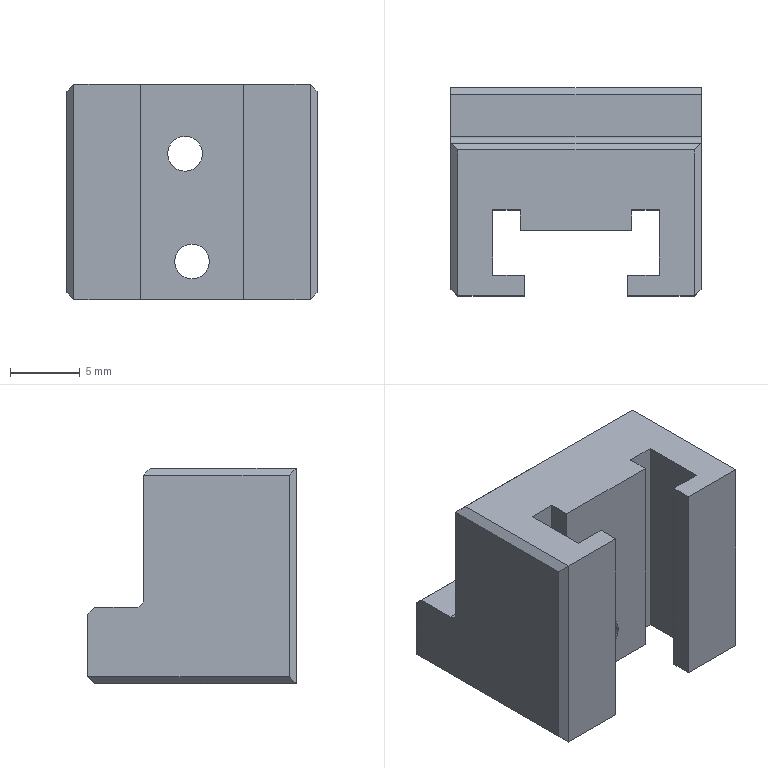Part | SolidWorks | features HoleWzd 2, Chamfer 1, Cut 1, Extrusion 1, Fillet 1 | 1 solid | 34 faces | box 18 x 15 x 15.5 mm | volume 2507 mm3 | plane 29 | cylinder 5 | commonest cylinder face diameters 2.5 x4 1 x1
STEP:
#1=CARTESIAN_POINT('',(0.,0.,-25.5));
#2=VERTEX_POINT('',#1);
#3=CARTESIAN_POINT('',(0.,0.,-28.));
#4=VERTEX_POINT('',#3);
#5=CARTESIAN_POINT('',(0.,0.,-26.75));
#6=DIRECTION('',(0.,-1.,0.));
#7=DIRECTION('',(1.,0.,0.));
#8=AXIS2_PLACEMENT_3D('',#5,#6,#7);
#9=CIRCLE('',#8,1.25);
#10=EDGE_CURVE('',#2,#4,#9,.T.);
#11=ORIENTED_EDGE('',*,*,#10,.T.);
#12=CARTESIAN_POINT('',(0.,10.3,-28.));
#13=VERTEX_POINT('',#12);
#14=CARTESIAN_POINT('',(0.,10.3,-28.));
#15=DIRECTION('',(0.,1.,0.));
#16=VECTOR('',#15,1000.);
#17=LINE('',#14,#16);
#18=EDGE_CURVE('',#4,#13,#17,.T.);
#19=ORIENTED_EDGE('',*,*,#18,.T.);
#20=CARTESIAN_POINT('',(0.,10.3,-25.5));
#21=VERTEX_POINT('',#20);
#22=CARTESIAN_POINT('',(0.,10.3,-26.75));
#23=DIRECTION('',(0.,1.,0.));
#24=DIRECTION('',(0.,0.,1.));
#25=AXIS2_PLACEMENT_3D('',#22,#23,#24);
#26=CIRCLE('',#25,1.25);
#27=EDGE_CURVE('',#13,#21,#26,.T.);
#28=ORIENTED_EDGE('',*,*,#27,.T.);
#29=CARTESIAN_POINT('',(0.,10.3,-25.5));
#30=DIRECTION('',(0.,1.,0.));
#31=VECTOR('',#30,1000.);
#32=LINE('',#29,#31);
#33=EDGE_CURVE('',#2,#21,#32,.T.);
#34=ORIENTED_EDGE('',*,*,#33,.F.);
#35=EDGE_LOOP('',(#11,#19,#28,#34));
#36=FACE_OUTER_BOUND('',#35,.T.);
#37=CARTESIAN_POINT('',(0.,10.3,-26.75));
#38=DIRECTION('',(0.,1.,0.));
#39=DIRECTION('',(0.,0.,1.));
#40=AXIS2_PLACEMENT_3D('',#37,#38,#39);
#41=CYLINDRICAL_SURFACE('',#40,1.25);
#42=ADVANCED_FACE('',(#36),#41,.F.);
#43=CARTESIAN_POINT('',(-0.5,0.,-17.75));
#44=VERTEX_POINT('',#43);
#45=CARTESIAN_POINT('',(-0.5,0.,-20.25));
#46=VERTEX_POINT('',#45);
#47=CARTESIAN_POINT('',(-0.5,0.,-19.));
#48=DIRECTION('',(0.,-1.,0.));
#49=DIRECTION('',(1.,0.,0.));
#50=AXIS2_PLACEMENT_3D('',#47,#48,#49);
#51=CIRCLE('',#50,1.25);
#52=EDGE_CURVE('',#44,#46,#51,.T.);
#53=ORIENTED_EDGE('',*,*,#52,.T.);
#54=CARTESIAN_POINT('',(-0.5,6.3,-20.25));
#55=VERTEX_POINT('',#54);
#56=CARTESIAN_POINT('',(-0.5,6.3,-20.25));
#57=DIRECTION('',(0.,1.,0.));
#58=VECTOR('',#57,1000.);
#59=LINE('',#56,#58);
#60=EDGE_CURVE('',#46,#55,#59,.T.);
#61=ORIENTED_EDGE('',*,*,#60,.T.);
#62=CARTESIAN_POINT('',(-0.5,6.3,-17.75));
#63=VERTEX_POINT('',#62);
#64=CARTESIAN_POINT('',(-0.5,6.3,-19.));
#65=DIRECTION('',(0.,1.,0.));
#66=DIRECTION('',(0.,0.,1.));
#67=AXIS2_PLACEMENT_3D('',#64,#65,#66);
#68=CIRCLE('',#67,1.25);
#69=EDGE_CURVE('',#55,#63,#68,.T.);
#70=ORIENTED_EDGE('',*,*,#69,.T.);
#71=CARTESIAN_POINT('',(-0.5,6.3,-17.75));
#72=DIRECTION('',(0.,1.,0.));
#73=VECTOR('',#72,1000.);
#74=LINE('',#71,#73);
#75=EDGE_CURVE('',#44,#63,#74,.T.);
#76=ORIENTED_EDGE('',*,*,#75,.F.);
#77=EDGE_LOOP('',(#53,#61,#70,#76));
#78=FACE_OUTER_BOUND('',#77,.T.);
#79=CARTESIAN_POINT('',(-0.5,6.3,-19.));
#80=DIRECTION('',(0.,1.,0.));
#81=DIRECTION('',(0.,0.,1.));
#82=AXIS2_PLACEMENT_3D('',#79,#80,#81);
#83=CYLINDRICAL_SURFACE('',#82,1.25);
#84=ADVANCED_FACE('',(#78),#83,.F.);
#85=CARTESIAN_POINT('',(3.7,-4.7,-29.5));
#86=VERTEX_POINT('',#85);
#87=CARTESIAN_POINT('',(8.5,-4.7,-29.5));
#88=VERTEX_POINT('',#87);
#89=CARTESIAN_POINT('',(3.7,-4.7,-29.5));
#90=DIRECTION('',(1.,0.,0.));
#91=VECTOR('',#90,1000.);
#92=LINE('',#89,#91);
#93=EDGE_CURVE('',#86,#88,#92,.T.);
#94=ORIENTED_EDGE('',*,*,#93,.T.);
#95=CARTESIAN_POINT('',(8.5,-4.7,-14.));
#96=VERTEX_POINT('',#95);
#97=CARTESIAN_POINT('',(8.5,-4.7,-29.5));
#98=DIRECTION('',(0.,0.,1.));
#99=VECTOR('',#98,1000.);
#100=LINE('',#97,#99);
#101=EDGE_CURVE('',#88,#96,#100,.T.);
#102=ORIENTED_EDGE('',*,*,#101,.T.);
#103=CARTESIAN_POINT('',(3.7,-4.7,-14.));
#104=VERTEX_POINT('',#103);
#105=CARTESIAN_POINT('',(3.7,-4.7,-14.));
#106=DIRECTION('',(1.,0.,0.));
#107=VECTOR('',#106,1000.);
#108=LINE('',#105,#107);
#109=EDGE_CURVE('',#104,#96,#108,.T.);
#110=ORIENTED_EDGE('',*,*,#109,.F.);
#111=CARTESIAN_POINT('',(3.7,-4.7,-29.5));
#112=DIRECTION('',(0.,0.,1.));
#113=VECTOR('',#112,1000.);
#114=LINE('',#111,#113);
#115=EDGE_CURVE('',#86,#104,#114,.T.);
#116=ORIENTED_EDGE('',*,*,#115,.F.);
#117=EDGE_LOOP('',(#94,#102,#110,#116));
#118=FACE_OUTER_BOUND('',#117,.T.);
#119=CARTESIAN_POINT('',(3.7,-4.7,-29.5));
#120=DIRECTION('',(0.,-1.,0.));
#121=DIRECTION('',(1.,0.,0.));
#122=AXIS2_PLACEMENT_3D('',#119,#120,#121);
#123=PLANE('',#122);
#124=ADVANCED_FACE('',(#118),#123,.T.);
#125=CARTESIAN_POINT('',(3.7,-3.2,-14.));
#126=VERTEX_POINT('',#125);
#127=CARTESIAN_POINT('',(3.7,-3.2,-14.));
#128=DIRECTION('',(0.,-1.,0.));
#129=VECTOR('',#128,1000.);
#130=LINE('',#127,#129);
#131=EDGE_CURVE('',#126,#104,#130,.T.);
#132=ORIENTED_EDGE('',*,*,#131,.F.);
#133=CARTESIAN_POINT('',(3.7,-3.2,-29.5));
#134=VERTEX_POINT('',#133);
#135=CARTESIAN_POINT('',(3.7,-3.2,-29.5));
#136=DIRECTION('',(0.,0.,1.));
#137=VECTOR('',#136,1000.);
#138=LINE('',#135,#137);
#139=EDGE_CURVE('',#134,#126,#138,.T.);
#140=ORIENTED_EDGE('',*,*,#139,.F.);
#141=CARTESIAN_POINT('',(3.7,-3.2,-29.5));
#142=DIRECTION('',(0.,-1.,0.));
#143=VECTOR('',#142,1000.);
#144=LINE('',#141,#143);
#145=EDGE_CURVE('',#134,#86,#144,.T.);
#146=ORIENTED_EDGE('',*,*,#145,.T.);
#147=ORIENTED_EDGE('',*,*,#115,.T.);
#148=EDGE_LOOP('',(#132,#140,#146,#147));
#149=FACE_OUTER_BOUND('',#148,.T.);
#150=CARTESIAN_POINT('',(3.7,-3.2,-29.5));
#151=DIRECTION('',(-1.,0.,0.));
#152=DIRECTION('',(0.,0.,1.));
#153=AXIS2_PLACEMENT_3D('',#150,#151,#152);
#154=PLANE('',#153);
#155=ADVANCED_FACE('',(#149),#154,.T.);
#156=CARTESIAN_POINT('',(6.,-3.2,-14.));
#157=VERTEX_POINT('',#156);
#158=CARTESIAN_POINT('',(6.,-3.2,-14.));
#159=DIRECTION('',(-1.,0.,0.));
#160=VECTOR('',#159,1000.);
#161=LINE('',#158,#160);
#162=EDGE_CURVE('',#157,#126,#161,.T.);
#163=ORIENTED_EDGE('',*,*,#162,.F.);
#164=CARTESIAN_POINT('',(6.,-3.2,-29.5));
#165=VERTEX_POINT('',#164);
#166=CARTESIAN_POINT('',(6.,-3.2,-29.5));
#167=DIRECTION('',(0.,0.,1.));
#168=VECTOR('',#167,1000.);
#169=LINE('',#166,#168);
#170=EDGE_CURVE('',#165,#157,#169,.T.);
#171=ORIENTED_EDGE('',*,*,#170,.F.);
#172=CARTESIAN_POINT('',(6.,-3.2,-29.5));
#173=DIRECTION('',(-1.,0.,0.));
#174=VECTOR('',#173,1000.);
#175=LINE('',#172,#174);
#176=EDGE_CURVE('',#165,#134,#175,.T.);
#177=ORIENTED_EDGE('',*,*,#176,.T.);
#178=ORIENTED_EDGE('',*,*,#139,.T.);
#179=EDGE_LOOP('',(#163,#171,#177,#178));
#180=FACE_OUTER_BOUND('',#179,.T.);
#181=CARTESIAN_POINT('',(6.,-3.2,-29.5));
#182=DIRECTION('',(0.,1.,0.));
#183=DIRECTION('',(0.,0.,1.));
#184=AXIS2_PLACEMENT_3D('',#181,#182,#183);
#185=PLANE('',#184);
#186=ADVANCED_FACE('',(#180),#185,.T.);
#187=CARTESIAN_POINT('',(6.,1.5,-14.));
#188=VERTEX_POINT('',#187);
#189=CARTESIAN_POINT('',(6.,1.5,-14.));
#190=DIRECTION('',(0.,-1.,0.));
#191=VECTOR('',#190,1000.);
#192=LINE('',#189,#191);
#193=EDGE_CURVE('',#188,#157,#192,.T.);
#194=ORIENTED_EDGE('',*,*,#193,.F.);
#195=CARTESIAN_POINT('',(6.,1.5,-29.5));
#196=VERTEX_POINT('',#195);
#197=CARTESIAN_POINT('',(6.,1.5,-29.5));
#198=DIRECTION('',(0.,0.,1.));
#199=VECTOR('',#198,1000.);
#200=LINE('',#197,#199);
#201=EDGE_CURVE('',#196,#188,#200,.T.);
#202=ORIENTED_EDGE('',*,*,#201,.F.);
#203=CARTESIAN_POINT('',(6.,1.5,-29.5));
#204=DIRECTION('',(0.,-1.,0.));
#205=VECTOR('',#204,1000.);
#206=LINE('',#203,#205);
#207=EDGE_CURVE('',#196,#165,#206,.T.);
#208=ORIENTED_EDGE('',*,*,#207,.T.);
#209=ORIENTED_EDGE('',*,*,#170,.T.);
#210=EDGE_LOOP('',(#194,#202,#208,#209));
#211=FACE_OUTER_BOUND('',#210,.T.);
#212=CARTESIAN_POINT('',(6.,1.5,-29.5));
#213=DIRECTION('',(-1.,0.,0.));
#214=DIRECTION('',(0.,-1.,0.));
#215=AXIS2_PLACEMENT_3D('',#212,#213,#214);
#216=PLANE('',#215);
#217=ADVANCED_FACE('',(#211),#216,.T.);
#218=CARTESIAN_POINT('',(4.,1.5,-14.));
#219=VERTEX_POINT('',#218);
#220=CARTESIAN_POINT('',(4.,1.5,-14.));
#221=DIRECTION('',(1.,0.,0.));
#222=VECTOR('',#221,1000.);
#223=LINE('',#220,#222);
#224=EDGE_CURVE('',#219,#188,#223,.T.);
#225=ORIENTED_EDGE('',*,*,#224,.F.);
#226=CARTESIAN_POINT('',(4.,1.5,-29.5));
#227=VERTEX_POINT('',#226);
#228=CARTESIAN_POINT('',(4.,1.5,-29.5));
#229=DIRECTION('',(0.,0.,1.));
#230=VECTOR('',#229,1000.);
#231=LINE('',#228,#230);
#232=EDGE_CURVE('',#227,#219,#231,.T.);
#233=ORIENTED_EDGE('',*,*,#232,.F.);
#234=CARTESIAN_POINT('',(4.,1.5,-29.5));
#235=DIRECTION('',(1.,0.,0.));
#236=VECTOR('',#235,1000.);
#237=LINE('',#234,#236);
#238=EDGE_CURVE('',#227,#196,#237,.T.);
#239=ORIENTED_EDGE('',*,*,#238,.T.);
#240=ORIENTED_EDGE('',*,*,#201,.T.);
#241=EDGE_LOOP('',(#225,#233,#239,#240));
#242=FACE_OUTER_BOUND('',#241,.T.);
#243=CARTESIAN_POINT('',(4.,1.5,-29.5));
#244=DIRECTION('',(0.,-1.,0.));
#245=DIRECTION('',(0.,0.,-1.));
#246=AXIS2_PLACEMENT_3D('',#243,#244,#245);
#247=PLANE('',#246);
#248=ADVANCED_FACE('',(#242),#247,.T.);
#249=CARTESIAN_POINT('',(4.,0.,-14.));
#250=VERTEX_POINT('',#249);
#251=CARTESIAN_POINT('',(4.,0.,-14.));
#252=DIRECTION('',(0.,1.,0.));
#253=VECTOR('',#252,1000.);
#254=LINE('',#251,#253);
#255=EDGE_CURVE('',#250,#219,#254,.T.);
#256=ORIENTED_EDGE('',*,*,#255,.F.);
#257=CARTESIAN_POINT('',(4.,0.,-29.5));
#258=VERTEX_POINT('',#257);
#259=CARTESIAN_POINT('',(4.,0.,-29.5));
#260=DIRECTION('',(0.,0.,1.));
#261=VECTOR('',#260,1000.);
#262=LINE('',#259,#261);
#263=EDGE_CURVE('',#258,#250,#262,.T.);
#264=ORIENTED_EDGE('',*,*,#263,.F.);
#265=CARTESIAN_POINT('',(4.,0.,-29.5));
#266=DIRECTION('',(0.,1.,0.));
#267=VECTOR('',#266,1000.);
#268=LINE('',#265,#267);
#269=EDGE_CURVE('',#258,#227,#268,.T.);
#270=ORIENTED_EDGE('',*,*,#269,.T.);
#271=ORIENTED_EDGE('',*,*,#232,.T.);
#272=EDGE_LOOP('',(#256,#264,#270,#271));
#273=FACE_OUTER_BOUND('',#272,.T.);
#274=CARTESIAN_POINT('',(4.,0.,-29.5));
#275=DIRECTION('',(1.,0.,0.));
#276=DIRECTION('',(0.,1.,0.));
#277=AXIS2_PLACEMENT_3D('',#274,#275,#276);
#278=PLANE('',#277);
#279=ADVANCED_FACE('',(#273),#278,.T.);
#280=ORIENTED_EDGE('',*,*,#10,.F.);
#281=CARTESIAN_POINT('',(0.,0.,-26.75));
#282=DIRECTION('',(0.,-1.,0.));
#283=DIRECTION('',(1.,0.,0.));
#284=AXIS2_PLACEMENT_3D('',#281,#282,#283);
#285=CIRCLE('',#284,1.25);
#286=EDGE_CURVE('',#4,#2,#285,.T.);
#287=ORIENTED_EDGE('',*,*,#286,.F.);
#288=EDGE_LOOP('',(#280,#287));
#289=FACE_BOUND('',#288,.T.);
#290=ORIENTED_EDGE('',*,*,#52,.F.);
#291=CARTESIAN_POINT('',(-0.5,0.,-19.));
#292=DIRECTION('',(0.,-1.,0.));
#293=DIRECTION('',(1.,0.,0.));
#294=AXIS2_PLACEMENT_3D('',#291,#292,#293);
#295=CIRCLE('',#294,1.25);
#296=EDGE_CURVE('',#46,#44,#295,.T.);
#297=ORIENTED_EDGE('',*,*,#296,.F.);
#298=EDGE_LOOP('',(#290,#297));
#299=FACE_BOUND('',#298,.T.);
#300=CARTESIAN_POINT('',(-4.,0.,-14.));
#301=VERTEX_POINT('',#300);
#302=CARTESIAN_POINT('',(0.,0.,-14.));
#303=DIRECTION('',(1.,0.,0.));
#304=VECTOR('',#303,1000.);
#305=LINE('',#302,#304);
#306=EDGE_CURVE('',#301,#250,#305,.T.);
#307=ORIENTED_EDGE('',*,*,#306,.F.);
#308=CARTESIAN_POINT('',(-4.,0.,-29.5));
#309=VERTEX_POINT('',#308);
#310=CARTESIAN_POINT('',(-4.,0.,-29.5));
#311=DIRECTION('',(0.,0.,1.));
#312=VECTOR('',#311,1000.);
#313=LINE('',#310,#312);
#314=EDGE_CURVE('',#309,#301,#313,.T.);
#315=ORIENTED_EDGE('',*,*,#314,.F.);
#316=CARTESIAN_POINT('',(-4.,0.,-29.5));
#317=DIRECTION('',(1.,0.,0.));
#318=VECTOR('',#317,1000.);
#319=LINE('',#316,#318);
#320=EDGE_CURVE('',#309,#258,#319,.T.);
#321=ORIENTED_EDGE('',*,*,#320,.T.);
#322=ORIENTED_EDGE('',*,*,#263,.T.);
#323=EDGE_LOOP('',(#307,#315,#321,#322));
#324=FACE_OUTER_BOUND('',#323,.T.);
#325=CARTESIAN_POINT('',(0.,0.,-29.5));
#326=DIRECTION('',(0.,-1.,0.));
#327=DIRECTION('',(1.,0.,0.));
#328=AXIS2_PLACEMENT_3D('',#325,#326,#327);
#329=PLANE('',#328);
#330=ADVANCED_FACE('',(#289,#299,#324),#329,.T.);
#331=CARTESIAN_POINT('',(-4.,1.5,-14.));
#332=VERTEX_POINT('',#331);
#333=CARTESIAN_POINT('',(-4.,1.5,-14.));
#334=DIRECTION('',(0.,-1.,0.));
#335=VECTOR('',#334,1000.);
#336=LINE('',#333,#335);
#337=EDGE_CURVE('',#332,#301,#336,.T.);
#338=ORIENTED_EDGE('',*,*,#337,.F.);
#339=CARTESIAN_POINT('',(-4.,1.5,-29.5));
#340=VERTEX_POINT('',#339);
#341=CARTESIAN_POINT('',(-4.,1.5,-29.5));
#342=DIRECTION('',(0.,0.,1.));
#343=VECTOR('',#342,1000.);
#344=LINE('',#341,#343);
#345=EDGE_CURVE('',#340,#332,#344,.T.);
#346=ORIENTED_EDGE('',*,*,#345,.F.);
#347=CARTESIAN_POINT('',(-4.,1.5,-29.5));
#348=DIRECTION('',(0.,-1.,0.));
#349=VECTOR('',#348,1000.);
#350=LINE('',#347,#349);
#351=EDGE_CURVE('',#340,#309,#350,.T.);
#352=ORIENTED_EDGE('',*,*,#351,.T.);
#353=ORIENTED_EDGE('',*,*,#314,.T.);
#354=EDGE_LOOP('',(#338,#346,#352,#353));
#355=FACE_OUTER_BOUND('',#354,.T.);
#356=CARTESIAN_POINT('',(-4.,1.5,-29.5));
#357=DIRECTION('',(-1.,0.,0.));
#358=DIRECTION('',(0.,-1.,0.));
#359=AXIS2_PLACEMENT_3D('',#356,#357,#358);
#360=PLANE('',#359);
#361=ADVANCED_FACE('',(#355),#360,.T.);
#362=CARTESIAN_POINT('',(-6.,1.5,-14.));
#363=VERTEX_POINT('',#362);
#364=CARTESIAN_POINT('',(-6.,1.5,-14.));
#365=DIRECTION('',(1.,0.,0.));
#366=VECTOR('',#365,1000.);
#367=LINE('',#364,#366);
#368=EDGE_CURVE('',#363,#332,#367,.T.);
#369=ORIENTED_EDGE('',*,*,#368,.F.);
#370=CARTESIAN_POINT('',(-6.,1.5,-29.5));
#371=VERTEX_POINT('',#370);
#372=CARTESIAN_POINT('',(-6.,1.5,-29.5));
#373=DIRECTION('',(0.,0.,1.));
#374=VECTOR('',#373,1000.);
#375=LINE('',#372,#374);
#376=EDGE_CURVE('',#371,#363,#375,.T.);
#377=ORIENTED_EDGE('',*,*,#376,.F.);
#378=CARTESIAN_POINT('',(-6.,1.5,-29.5));
#379=DIRECTION('',(1.,0.,0.));
#380=VECTOR('',#379,1000.);
#381=LINE('',#378,#380);
#382=EDGE_CURVE('',#371,#340,#381,.T.);
#383=ORIENTED_EDGE('',*,*,#382,.T.);
#384=ORIENTED_EDGE('',*,*,#345,.T.);
#385=EDGE_LOOP('',(#369,#377,#383,#384));
#386=FACE_OUTER_BOUND('',#385,.T.);
#387=CARTESIAN_POINT('',(-6.,1.5,-29.5));
#388=DIRECTION('',(0.,-1.,0.));
#389=DIRECTION('',(0.,0.,-1.));
#390=AXIS2_PLACEMENT_3D('',#387,#388,#389);
#391=PLANE('',#390);
#392=ADVANCED_FACE('',(#386),#391,.T.);
#393=CARTESIAN_POINT('',(-6.,-3.2,-14.));
#394=VERTEX_POINT('',#393);
#395=CARTESIAN_POINT('',(-6.,-3.2,-14.));
#396=DIRECTION('',(0.,1.,0.));
#397=VECTOR('',#396,1000.);
#398=LINE('',#395,#397);
#399=EDGE_CURVE('',#394,#363,#398,.T.);
#400=ORIENTED_EDGE('',*,*,#399,.F.);
#401=CARTESIAN_POINT('',(-6.,-3.2,-29.5));
#402=VERTEX_POINT('',#401);
#403=CARTESIAN_POINT('',(-6.,-3.2,-29.5));
#404=DIRECTION('',(0.,0.,1.));
#405=VECTOR('',#404,1000.);
#406=LINE('',#403,#405);
#407=EDGE_CURVE('',#402,#394,#406,.T.);
#408=ORIENTED_EDGE('',*,*,#407,.F.);
#409=CARTESIAN_POINT('',(-6.,-3.2,-29.5));
#410=DIRECTION('',(0.,1.,0.));
#411=VECTOR('',#410,1000.);
#412=LINE('',#409,#411);
#413=EDGE_CURVE('',#402,#371,#412,.T.);
#414=ORIENTED_EDGE('',*,*,#413,.T.);
#415=ORIENTED_EDGE('',*,*,#376,.T.);
#416=EDGE_LOOP('',(#400,#408,#414,#415));
#417=FACE_OUTER_BOUND('',#416,.T.);
#418=CARTESIAN_POINT('',(-6.,-3.2,-29.5));
#419=DIRECTION('',(1.,0.,0.));
#420=DIRECTION('',(0.,1.,0.));
#421=AXIS2_PLACEMENT_3D('',#418,#419,#420);
#422=PLANE('',#421);
#423=ADVANCED_FACE('',(#417),#422,.T.);
#424=CARTESIAN_POINT('',(-3.7,-3.2,-14.));
#425=VERTEX_POINT('',#424);
#426=CARTESIAN_POINT('',(-3.7,-3.2,-14.));
#427=DIRECTION('',(-1.,0.,0.));
#428=VECTOR('',#427,1000.);
#429=LINE('',#426,#428);
#430=EDGE_CURVE('',#425,#394,#429,.T.);
#431=ORIENTED_EDGE('',*,*,#430,.F.);
#432=CARTESIAN_POINT('',(-3.7,-3.2,-29.5));
#433=VERTEX_POINT('',#432);
#434=CARTESIAN_POINT('',(-3.7,-3.2,-29.5));
#435=DIRECTION('',(0.,0.,1.));
#436=VECTOR('',#435,1000.);
#437=LINE('',#434,#436);
#438=EDGE_CURVE('',#433,#425,#437,.T.);
#439=ORIENTED_EDGE('',*,*,#438,.F.);
#440=CARTESIAN_POINT('',(-3.7,-3.2,-29.5));
#441=DIRECTION('',(-1.,0.,0.));
#442=VECTOR('',#441,1000.);
#443=LINE('',#440,#442);
#444=EDGE_CURVE('',#433,#402,#443,.T.);
#445=ORIENTED_EDGE('',*,*,#444,.T.);
#446=ORIENTED_EDGE('',*,*,#407,.T.);
#447=EDGE_LOOP('',(#431,#439,#445,#446));
#448=FACE_OUTER_BOUND('',#447,.T.);
#449=CARTESIAN_POINT('',(-3.7,-3.2,-29.5));
#450=DIRECTION('',(0.,1.,0.));
#451=DIRECTION('',(0.,0.,1.));
#452=AXIS2_PLACEMENT_3D('',#449,#450,#451);
#453=PLANE('',#452);
#454=ADVANCED_FACE('',(#448),#453,.T.);
#455=CARTESIAN_POINT('',(-3.7,-4.7,-14.));
#456=VERTEX_POINT('',#455);
#457=CARTESIAN_POINT('',(-3.7,-3.2,-14.));
#458=DIRECTION('',(0.,-1.,0.));
#459=VECTOR('',#458,1000.);
#460=LINE('',#457,#459);
#461=EDGE_CURVE('',#425,#456,#460,.T.);
#462=ORIENTED_EDGE('',*,*,#461,.T.);
#463=CARTESIAN_POINT('',(-3.7,-4.7,-29.5));
#464=VERTEX_POINT('',#463);
#465=CARTESIAN_POINT('',(-3.7,-4.7,-29.5));
#466=DIRECTION('',(0.,0.,1.));
#467=VECTOR('',#466,1000.);
#468=LINE('',#465,#467);
#469=EDGE_CURVE('',#464,#456,#468,.T.);
#470=ORIENTED_EDGE('',*,*,#469,.F.);
#471=CARTESIAN_POINT('',(-3.7,-3.2,-29.5));
#472=DIRECTION('',(0.,-1.,0.));
#473=VECTOR('',#472,1000.);
#474=LINE('',#471,#473);
#475=EDGE_CURVE('',#433,#464,#474,.T.);
#476=ORIENTED_EDGE('',*,*,#475,.F.);
#477=ORIENTED_EDGE('',*,*,#438,.T.);
#478=EDGE_LOOP('',(#462,#470,#476,#477));
#479=FACE_OUTER_BOUND('',#478,.T.);
#480=CARTESIAN_POINT('',(-3.7,-3.2,-29.5));
#481=DIRECTION('',(-1.,0.,0.));
#482=DIRECTION('',(0.,0.,1.));
#483=AXIS2_PLACEMENT_3D('',#480,#481,#482);
#484=PLANE('',#483);
#485=ADVANCED_FACE('',(#479),#484,.F.);
#486=CARTESIAN_POINT('',(-8.5,-4.7,-14.));
#487=VERTEX_POINT('',#486);
#488=CARTESIAN_POINT('',(-3.7,-4.7,-14.));
#489=DIRECTION('',(-1.,0.,0.));
#490=VECTOR('',#489,1000.);
#491=LINE('',#488,#490);
#492=EDGE_CURVE('',#456,#487,#491,.T.);
#493=ORIENTED_EDGE('',*,*,#492,.T.);
#494=CARTESIAN_POINT('',(-8.5,-4.7,-29.5));
#495=VERTEX_POINT('',#494);
#496=CARTESIAN_POINT('',(-8.5,-4.7,-29.5));
#497=DIRECTION('',(0.,0.,-1.));
#498=VECTOR('',#497,1000.);
#499=LINE('',#496,#498);
#500=EDGE_CURVE('',#487,#495,#499,.T.);
#501=ORIENTED_EDGE('',*,*,#500,.T.);
#502=CARTESIAN_POINT('',(-3.7,-4.7,-29.5));
#503=DIRECTION('',(-1.,0.,0.));
#504=VECTOR('',#503,1000.);
#505=LINE('',#502,#504);
#506=EDGE_CURVE('',#464,#495,#505,.T.);
#507=ORIENTED_EDGE('',*,*,#506,.F.);
#508=ORIENTED_EDGE('',*,*,#469,.T.);
#509=EDGE_LOOP('',(#493,#501,#507,#508));
#510=FACE_OUTER_BOUND('',#509,.T.);
#511=CARTESIAN_POINT('',(-3.7,-4.7,-29.5));
#512=DIRECTION('',(0.,1.,0.));
#513=DIRECTION('',(-1.,0.,0.));
#514=AXIS2_PLACEMENT_3D('',#511,#512,#513);
#515=PLANE('',#514);
#516=ADVANCED_FACE('',(#510),#515,.F.);
#517=CARTESIAN_POINT('',(-9.,6.3,-14.5));
#518=VERTEX_POINT('',#517);
#519=CARTESIAN_POINT('',(-9.,6.3,-23.5));
#520=VERTEX_POINT('',#519);
#521=CARTESIAN_POINT('',(-9.,6.3,-14.));
#522=DIRECTION('',(0.,0.,-1.));
#523=VECTOR('',#522,1000.);
#524=LINE('',#521,#523);
#525=EDGE_CURVE('',#518,#520,#524,.T.);
#526=ORIENTED_EDGE('',*,*,#525,.T.);
#527=CARTESIAN_POINT('',(-9.,6.8,-24.));
#528=VERTEX_POINT('',#527);
#529=CARTESIAN_POINT('',(-9.,6.8,-23.5));
#530=DIRECTION('',(1.,0.,0.));
#531=DIRECTION('',(0.,1.,0.));
#532=AXIS2_PLACEMENT_3D('',#529,#530,#531);
#533=CIRCLE('',#532,0.5);
#534=EDGE_CURVE('',#520,#528,#533,.T.);
#535=ORIENTED_EDGE('',*,*,#534,.T.);
#536=CARTESIAN_POINT('',(-9.,9.8,-24.));
#537=VERTEX_POINT('',#536);
#538=CARTESIAN_POINT('',(-9.,6.3,-24.));
#539=DIRECTION('',(0.,1.,0.));
#540=VECTOR('',#539,1000.);
#541=LINE('',#538,#540);
#542=EDGE_CURVE('',#528,#537,#541,.T.);
#543=ORIENTED_EDGE('',*,*,#542,.T.);
#544=CARTESIAN_POINT('',(-9.,10.3,-24.5));
#545=VERTEX_POINT('',#544);
#546=CARTESIAN_POINT('',(-9.,10.3,-24.5));
#547=DIRECTION('',(0.,0.7071,-0.7071));
#548=VECTOR('',#547,1000.);
#549=LINE('',#546,#548);
#550=EDGE_CURVE('',#537,#545,#549,.T.);
#551=ORIENTED_EDGE('',*,*,#550,.T.);
#552=CARTESIAN_POINT('',(-9.,10.3,-29.));
#553=VERTEX_POINT('',#552);
#554=CARTESIAN_POINT('',(-9.,10.3,-29.5));
#555=DIRECTION('',(0.,0.,1.));
#556=VECTOR('',#555,1000.);
#557=LINE('',#554,#556);
#558=EDGE_CURVE('',#553,#545,#557,.T.);
#559=ORIENTED_EDGE('',*,*,#558,.F.);
#560=CARTESIAN_POINT('',(-9.,-4.2,-29.));
#561=VERTEX_POINT('',#560);
#562=CARTESIAN_POINT('',(-9.,-4.7,-29.));
#563=DIRECTION('',(0.,-1.,0.));
#564=VECTOR('',#563,1000.);
#565=LINE('',#562,#564);
#566=EDGE_CURVE('',#553,#561,#565,.T.);
#567=ORIENTED_EDGE('',*,*,#566,.T.);
#568=CARTESIAN_POINT('',(-9.,-4.2,-14.5));
#569=VERTEX_POINT('',#568);
#570=CARTESIAN_POINT('',(-9.,-4.2,-29.5));
#571=DIRECTION('',(0.,0.,1.));
#572=VECTOR('',#571,1000.);
#573=LINE('',#570,#572);
#574=EDGE_CURVE('',#561,#569,#573,.T.);
#575=ORIENTED_EDGE('',*,*,#574,.T.);
#576=CARTESIAN_POINT('',(-9.,6.3,-14.5));
#577=DIRECTION('',(0.,1.,0.));
#578=VECTOR('',#577,1000.);
#579=LINE('',#576,#578);
#580=EDGE_CURVE('',#569,#518,#579,.T.);
#581=ORIENTED_EDGE('',*,*,#580,.T.);
#582=EDGE_LOOP('',(#526,#535,#543,#551,#559,#567,#575,#581));
#583=FACE_OUTER_BOUND('',#582,.T.);
#584=CARTESIAN_POINT('',(-9.,-4.7,-29.5));
#585=DIRECTION('',(1.,0.,0.));
#586=DIRECTION('',(0.,1.,0.));
#587=AXIS2_PLACEMENT_3D('',#584,#585,#586);
#588=PLANE('',#587);
#589=ADVANCED_FACE('',(#583),#588,.F.);
#590=CARTESIAN_POINT('',(0.,10.3,-26.75));
#591=DIRECTION('',(0.,1.,0.));
#592=DIRECTION('',(0.,0.,1.));
#593=AXIS2_PLACEMENT_3D('',#590,#591,#592);
#594=CIRCLE('',#593,1.25);
#595=EDGE_CURVE('',#21,#13,#594,.T.);
#596=ORIENTED_EDGE('',*,*,#595,.F.);
#597=ORIENTED_EDGE('',*,*,#27,.F.);
#598=EDGE_LOOP('',(#596,#597));
#599=FACE_BOUND('',#598,.T.);
#600=ORIENTED_EDGE('',*,*,#558,.T.);
#601=CARTESIAN_POINT('',(9.,10.3,-24.5));
#602=VERTEX_POINT('',#601);
#603=CARTESIAN_POINT('',(-9.,10.3,-24.5));
#604=DIRECTION('',(1.,0.,0.));
#605=VECTOR('',#604,1000.);
#606=LINE('',#603,#605);
#607=EDGE_CURVE('',#545,#602,#606,.T.);
#608=ORIENTED_EDGE('',*,*,#607,.T.);
#609=CARTESIAN_POINT('',(9.,10.3,-29.));
#610=VERTEX_POINT('',#609);
#611=CARTESIAN_POINT('',(9.,10.3,-29.5));
#612=DIRECTION('',(0.,0.,1.));
#613=VECTOR('',#612,1000.);
#614=LINE('',#611,#613);
#615=EDGE_CURVE('',#610,#602,#614,.T.);
#616=ORIENTED_EDGE('',*,*,#615,.F.);
#617=CARTESIAN_POINT('',(-9.,10.3,-29.));
#618=DIRECTION('',(-1.,0.,0.));
#619=VECTOR('',#618,1000.);
#620=LINE('',#617,#619);
#621=EDGE_CURVE('',#610,#553,#620,.T.);
#622=ORIENTED_EDGE('',*,*,#621,.T.);
#623=EDGE_LOOP('',(#600,#608,#616,#622));
#624=FACE_OUTER_BOUND('',#623,.T.);
#625=CARTESIAN_POINT('',(-9.,10.3,-29.5));
#626=DIRECTION('',(0.,-1.,0.));
#627=DIRECTION('',(0.,0.,-1.));
#628=AXIS2_PLACEMENT_3D('',#625,#626,#627);
#629=PLANE('',#628);
#630=ADVANCED_FACE('',(#599,#624),#629,.F.);
#631=ORIENTED_EDGE('',*,*,#615,.T.);
#632=CARTESIAN_POINT('',(9.,9.8,-24.));
#633=VERTEX_POINT('',#632);
#634=CARTESIAN_POINT('',(9.,5.3,-19.5));
#635=DIRECTION('',(0.,-0.7071,0.7071));
#636=VECTOR('',#635,1000.);
#637=LINE('',#634,#636);
#638=EDGE_CURVE('',#602,#633,#637,.T.);
#639=ORIENTED_EDGE('',*,*,#638,.T.);
#640=CARTESIAN_POINT('',(9.,6.8,-24.));
#641=VERTEX_POINT('',#640);
#642=CARTESIAN_POINT('',(9.,6.3,-24.));
#643=DIRECTION('',(0.,1.,0.));
#644=VECTOR('',#643,1000.);
#645=LINE('',#642,#644);
#646=EDGE_CURVE('',#641,#633,#645,.T.);
#647=ORIENTED_EDGE('',*,*,#646,.F.);
#648=CARTESIAN_POINT('',(9.,6.3,-23.5));
#649=VERTEX_POINT('',#648);
#650=CARTESIAN_POINT('',(9.,6.8,-23.5));
#651=DIRECTION('',(-1.,0.,0.));
#652=DIRECTION('',(0.,1.,0.));
#653=AXIS2_PLACEMENT_3D('',#650,#651,#652);
#654=CIRCLE('',#653,0.5);
#655=EDGE_CURVE('',#641,#649,#654,.T.);
#656=ORIENTED_EDGE('',*,*,#655,.T.);
#657=CARTESIAN_POINT('',(9.,6.3,-14.5));
#658=VERTEX_POINT('',#657);
#659=CARTESIAN_POINT('',(9.,6.3,-14.));
#660=DIRECTION('',(0.,0.,-1.));
#661=VECTOR('',#660,1000.);
#662=LINE('',#659,#661);
#663=EDGE_CURVE('',#658,#649,#662,.T.);
#664=ORIENTED_EDGE('',*,*,#663,.F.);
#665=CARTESIAN_POINT('',(9.,-4.2,-14.5));
#666=VERTEX_POINT('',#665);
#667=CARTESIAN_POINT('',(9.,-4.7,-14.5));
#668=DIRECTION('',(0.,-1.,0.));
#669=VECTOR('',#668,1000.);
#670=LINE('',#667,#669);
#671=EDGE_CURVE('',#658,#666,#670,.T.);
#672=ORIENTED_EDGE('',*,*,#671,.T.);
#673=CARTESIAN_POINT('',(9.,-4.2,-29.));
#674=VERTEX_POINT('',#673);
#675=CARTESIAN_POINT('',(9.,-4.2,-29.5));
#676=DIRECTION('',(0.,0.,-1.));
#677=VECTOR('',#676,1000.);
#678=LINE('',#675,#677);
#679=EDGE_CURVE('',#666,#674,#678,.T.);
#680=ORIENTED_EDGE('',*,*,#679,.T.);
#681=CARTESIAN_POINT('',(9.,10.3,-29.));
#682=DIRECTION('',(0.,1.,0.));
#683=VECTOR('',#682,1000.);
#684=LINE('',#681,#683);
#685=EDGE_CURVE('',#674,#610,#684,.T.);
#686=ORIENTED_EDGE('',*,*,#685,.T.);
#687=EDGE_LOOP('',(#631,#639,#647,#656,#664,#672,#680,#686));
#688=FACE_OUTER_BOUND('',#687,.T.);
#689=CARTESIAN_POINT('',(9.,-4.7,-29.5));
#690=DIRECTION('',(1.,0.,0.));
#691=DIRECTION('',(0.,1.,0.));
#692=AXIS2_PLACEMENT_3D('',#689,#690,#691);
#693=PLANE('',#692);
#694=ADVANCED_FACE('',(#688),#693,.T.);
#695=ORIENTED_EDGE('',*,*,#506,.T.);
#696=CARTESIAN_POINT('',(-8.5,9.8,-29.5));
#697=VERTEX_POINT('',#696);
#698=CARTESIAN_POINT('',(-8.5,0.,-29.5));
#699=DIRECTION('',(0.,1.,0.));
#700=VECTOR('',#699,1000.);
#701=LINE('',#698,#700);
#702=EDGE_CURVE('',#495,#697,#701,.T.);
#703=ORIENTED_EDGE('',*,*,#702,.T.);
#704=CARTESIAN_POINT('',(8.5,9.8,-29.5));
#705=VERTEX_POINT('',#704);
#706=CARTESIAN_POINT('',(0.,9.8,-29.5));
#707=DIRECTION('',(1.,0.,0.));
#708=VECTOR('',#707,1000.);
#709=LINE('',#706,#708);
#710=EDGE_CURVE('',#697,#705,#709,.T.);
#711=ORIENTED_EDGE('',*,*,#710,.T.);
#712=CARTESIAN_POINT('',(8.5,-4.7,-29.5));
#713=DIRECTION('',(0.,-1.,0.));
#714=VECTOR('',#713,1000.);
#715=LINE('',#712,#714);
#716=EDGE_CURVE('',#705,#88,#715,.T.);
#717=ORIENTED_EDGE('',*,*,#716,.T.);
#718=ORIENTED_EDGE('',*,*,#93,.F.);
#719=ORIENTED_EDGE('',*,*,#145,.F.);
#720=ORIENTED_EDGE('',*,*,#176,.F.);
#721=ORIENTED_EDGE('',*,*,#207,.F.);
#722=ORIENTED_EDGE('',*,*,#238,.F.);
#723=ORIENTED_EDGE('',*,*,#269,.F.);
#724=ORIENTED_EDGE('',*,*,#320,.F.);
#725=ORIENTED_EDGE('',*,*,#351,.F.);
#726=ORIENTED_EDGE('',*,*,#382,.F.);
#727=ORIENTED_EDGE('',*,*,#413,.F.);
#728=ORIENTED_EDGE('',*,*,#444,.F.);
#729=ORIENTED_EDGE('',*,*,#475,.T.);
#730=EDGE_LOOP('',(#695,#703,#711,#717,#718,#719,#720,#721,#722,#723,#724,#725,#726,#727,#728,#729));
#731=FACE_OUTER_BOUND('',#730,.T.);
#732=CARTESIAN_POINT('',(0.,0.,-29.5));
#733=DIRECTION('',(0.,0.,1.));
#734=DIRECTION('',(1.,0.,0.));
#735=AXIS2_PLACEMENT_3D('',#732,#733,#734);
#736=PLANE('',#735);
#737=ADVANCED_FACE('',(#731),#736,.F.);
#738=CARTESIAN_POINT('',(8.5,5.8,-14.));
#739=VERTEX_POINT('',#738);
#740=CARTESIAN_POINT('',(-8.5,5.8,-14.));
#741=VERTEX_POINT('',#740);
#742=CARTESIAN_POINT('',(-9.,5.8,-14.));
#743=DIRECTION('',(-1.,0.,0.));
#744=VECTOR('',#743,1000.);
#745=LINE('',#742,#744);
#746=EDGE_CURVE('',#739,#741,#745,.T.);
#747=ORIENTED_EDGE('',*,*,#746,.T.);
#748=CARTESIAN_POINT('',(-8.5,-4.7,-14.));
#749=DIRECTION('',(0.,-1.,0.));
#750=VECTOR('',#749,1000.);
#751=LINE('',#748,#750);
#752=EDGE_CURVE('',#741,#487,#751,.T.);
#753=ORIENTED_EDGE('',*,*,#752,.T.);
#754=ORIENTED_EDGE('',*,*,#492,.F.);
#755=ORIENTED_EDGE('',*,*,#461,.F.);
#756=ORIENTED_EDGE('',*,*,#430,.T.);
#757=ORIENTED_EDGE('',*,*,#399,.T.);
#758=ORIENTED_EDGE('',*,*,#368,.T.);
#759=ORIENTED_EDGE('',*,*,#337,.T.);
#760=ORIENTED_EDGE('',*,*,#306,.T.);
#761=ORIENTED_EDGE('',*,*,#255,.T.);
#762=ORIENTED_EDGE('',*,*,#224,.T.);
#763=ORIENTED_EDGE('',*,*,#193,.T.);
#764=ORIENTED_EDGE('',*,*,#162,.T.);
#765=ORIENTED_EDGE('',*,*,#131,.T.);
#766=ORIENTED_EDGE('',*,*,#109,.T.);
#767=CARTESIAN_POINT('',(8.5,0.,-14.));
#768=DIRECTION('',(0.,1.,0.));
#769=VECTOR('',#768,1000.);
#770=LINE('',#767,#769);
#771=EDGE_CURVE('',#96,#739,#770,.T.);
#772=ORIENTED_EDGE('',*,*,#771,.T.);
#773=EDGE_LOOP('',(#747,#753,#754,#755,#756,#757,#758,#759,#760,#761,#762,#763,#764,#765,#766,#772));
#774=FACE_OUTER_BOUND('',#773,.T.);
#775=CARTESIAN_POINT('',(0.,0.,-14.));
#776=DIRECTION('',(0.,0.,1.));
#777=DIRECTION('',(1.,0.,0.));
#778=AXIS2_PLACEMENT_3D('',#775,#776,#777);
#779=PLANE('',#778);
#780=ADVANCED_FACE('',(#774),#779,.T.);
#781=ORIENTED_EDGE('',*,*,#542,.F.);
#782=CARTESIAN_POINT('',(9.,6.8,-24.));
#783=DIRECTION('',(1.,0.,0.));
#784=VECTOR('',#783,1000.);
#785=LINE('',#782,#784);
#786=EDGE_CURVE('',#528,#641,#785,.T.);
#787=ORIENTED_EDGE('',*,*,#786,.T.);
#788=ORIENTED_EDGE('',*,*,#646,.T.);
#789=CARTESIAN_POINT('',(-9.,9.8,-24.));
#790=DIRECTION('',(-1.,0.,0.));
#791=VECTOR('',#790,1000.);
#792=LINE('',#789,#791);
#793=EDGE_CURVE('',#633,#537,#792,.T.);
#794=ORIENTED_EDGE('',*,*,#793,.T.);
#795=EDGE_LOOP('',(#781,#787,#788,#794));
#796=FACE_OUTER_BOUND('',#795,.T.);
#797=CARTESIAN_POINT('',(-9.,6.3,-24.));
#798=DIRECTION('',(0.,0.,-1.));
#799=DIRECTION('',(-1.,0.,0.));
#800=AXIS2_PLACEMENT_3D('',#797,#798,#799);
#801=PLANE('',#800);
#802=ADVANCED_FACE('',(#796),#801,.F.);
#803=CARTESIAN_POINT('',(-0.5,6.3,-19.));
#804=DIRECTION('',(0.,1.,0.));
#805=DIRECTION('',(0.,0.,1.));
#806=AXIS2_PLACEMENT_3D('',#803,#804,#805);
#807=CIRCLE('',#806,1.25);
#808=EDGE_CURVE('',#63,#55,#807,.T.);
#809=ORIENTED_EDGE('',*,*,#808,.F.);
#810=ORIENTED_EDGE('',*,*,#69,.F.);
#811=EDGE_LOOP('',(#809,#810));
#812=FACE_BOUND('',#811,.T.);
#813=ORIENTED_EDGE('',*,*,#663,.T.);
#814=CARTESIAN_POINT('',(-9.,6.3,-23.5));
#815=DIRECTION('',(-1.,0.,0.));
#816=VECTOR('',#815,1000.);
#817=LINE('',#814,#816);
#818=EDGE_CURVE('',#649,#520,#817,.T.);
#819=ORIENTED_EDGE('',*,*,#818,.T.);
#820=ORIENTED_EDGE('',*,*,#525,.F.);
#821=CARTESIAN_POINT('',(9.,6.3,-14.5));
#822=DIRECTION('',(1.,0.,0.));
#823=VECTOR('',#822,1000.);
#824=LINE('',#821,#823);
#825=EDGE_CURVE('',#518,#658,#824,.T.);
#826=ORIENTED_EDGE('',*,*,#825,.T.);
#827=EDGE_LOOP('',(#813,#819,#820,#826));
#828=FACE_OUTER_BOUND('',#827,.T.);
#829=CARTESIAN_POINT('',(-9.,6.3,-14.));
#830=DIRECTION('',(0.,-1.,0.));
#831=DIRECTION('',(1.,0.,0.));
#832=AXIS2_PLACEMENT_3D('',#829,#830,#831);
#833=PLANE('',#832);
#834=ADVANCED_FACE('',(#812,#828),#833,.F.);
#835=ORIENTED_EDGE('',*,*,#60,.F.);
#836=ORIENTED_EDGE('',*,*,#296,.T.);
#837=ORIENTED_EDGE('',*,*,#75,.T.);
#838=ORIENTED_EDGE('',*,*,#808,.T.);
#839=EDGE_LOOP('',(#835,#836,#837,#838));
#840=FACE_OUTER_BOUND('',#839,.T.);
#841=CARTESIAN_POINT('',(-0.5,6.3,-19.));
#842=DIRECTION('',(0.,1.,0.));
#843=DIRECTION('',(0.,0.,1.));
#844=AXIS2_PLACEMENT_3D('',#841,#842,#843);
#845=CYLINDRICAL_SURFACE('',#844,1.25);
#846=ADVANCED_FACE('',(#840),#845,.F.);
#847=ORIENTED_EDGE('',*,*,#18,.F.);
#848=ORIENTED_EDGE('',*,*,#286,.T.);
#849=ORIENTED_EDGE('',*,*,#33,.T.);
#850=ORIENTED_EDGE('',*,*,#595,.T.);
#851=EDGE_LOOP('',(#847,#848,#849,#850));
#852=FACE_OUTER_BOUND('',#851,.T.);
#853=CARTESIAN_POINT('',(0.,10.3,-26.75));
#854=DIRECTION('',(0.,1.,0.));
#855=DIRECTION('',(0.,0.,1.));
#856=AXIS2_PLACEMENT_3D('',#853,#854,#855);
#857=CYLINDRICAL_SURFACE('',#856,1.25);
#858=ADVANCED_FACE('',(#852),#857,.F.);
#859=ORIENTED_EDGE('',*,*,#550,.F.);
#860=ORIENTED_EDGE('',*,*,#793,.F.);
#861=ORIENTED_EDGE('',*,*,#638,.F.);
#862=ORIENTED_EDGE('',*,*,#607,.F.);
#863=EDGE_LOOP('',(#859,#860,#861,#862));
#864=FACE_OUTER_BOUND('',#863,.T.);
#865=CARTESIAN_POINT('',(-9.,10.3,-24.5));
#866=DIRECTION('',(0.,-0.7071,-0.7071));
#867=DIRECTION('',(1.,0.,0.));
#868=AXIS2_PLACEMENT_3D('',#865,#866,#867);
#869=PLANE('',#868);
#870=ADVANCED_FACE('',(#864),#869,.F.);
#871=CARTESIAN_POINT('',(4.,5.3,-34.));
#872=DIRECTION('',(0.5774,0.5774,0.5774));
#873=VECTOR('',#872,1000.);
#874=LINE('',#871,#873);
#875=EDGE_CURVE('',#705,#610,#874,.T.);
#876=ORIENTED_EDGE('',*,*,#875,.F.);
#877=ORIENTED_EDGE('',*,*,#710,.F.);
#878=CARTESIAN_POINT('',(-5.667,6.967,-32.333));
#879=DIRECTION('',(0.5774,-0.5774,-0.5774));
#880=VECTOR('',#879,1000.);
#881=LINE('',#878,#880);
#882=EDGE_CURVE('',#553,#697,#881,.T.);
#883=ORIENTED_EDGE('',*,*,#882,.F.);
#884=ORIENTED_EDGE('',*,*,#621,.F.);
#885=EDGE_LOOP('',(#876,#877,#883,#884));
#886=FACE_OUTER_BOUND('',#885,.T.);
#887=CARTESIAN_POINT('',(0.,9.8,-29.5));
#888=DIRECTION('',(0.,-0.7071,0.7071));
#889=DIRECTION('',(1.,0.,0.));
#890=AXIS2_PLACEMENT_3D('',#887,#888,#889);
#891=PLANE('',#890);
#892=ADVANCED_FACE('',(#886),#891,.F.);
#893=ORIENTED_EDGE('',*,*,#882,.T.);
#894=ORIENTED_EDGE('',*,*,#702,.F.);
#895=CARTESIAN_POINT('',(-10.067,-3.133,-27.933));
#896=DIRECTION('',(0.5774,-0.5774,-0.5774));
#897=VECTOR('',#896,1000.);
#898=LINE('',#895,#897);
#899=EDGE_CURVE('',#561,#495,#898,.T.);
#900=ORIENTED_EDGE('',*,*,#899,.F.);
#901=ORIENTED_EDGE('',*,*,#566,.F.);
#902=EDGE_LOOP('',(#893,#894,#900,#901));
#903=FACE_OUTER_BOUND('',#902,.T.);
#904=CARTESIAN_POINT('',(-8.5,0.,-29.5));
#905=DIRECTION('',(0.7071,0.,0.7071));
#906=DIRECTION('',(0.,1.,0.));
#907=AXIS2_PLACEMENT_3D('',#904,#905,#906);
#908=PLANE('',#907);
#909=ADVANCED_FACE('',(#903),#908,.F.);
#910=ORIENTED_EDGE('',*,*,#875,.T.);
#911=ORIENTED_EDGE('',*,*,#685,.F.);
#912=CARTESIAN_POINT('',(8.833,-4.367,-29.167));
#913=DIRECTION('',(0.5774,0.5774,0.5774));
#914=VECTOR('',#913,1000.);
#915=LINE('',#912,#914);
#916=EDGE_CURVE('',#88,#674,#915,.T.);
#917=ORIENTED_EDGE('',*,*,#916,.F.);
#918=ORIENTED_EDGE('',*,*,#716,.F.);
#919=EDGE_LOOP('',(#910,#911,#917,#918));
#920=FACE_OUTER_BOUND('',#919,.T.);
#921=CARTESIAN_POINT('',(9.,-4.7,-29.));
#922=DIRECTION('',(0.7071,0.,-0.7071));
#923=DIRECTION('',(0.,-1.,0.));
#924=AXIS2_PLACEMENT_3D('',#921,#922,#923);
#925=PLANE('',#924);
#926=ADVANCED_FACE('',(#920),#925,.T.);
#927=ORIENTED_EDGE('',*,*,#899,.T.);
#928=ORIENTED_EDGE('',*,*,#500,.F.);
#929=CARTESIAN_POINT('',(-14.,0.8,-19.5));
#930=DIRECTION('',(0.5774,-0.5774,0.5774));
#931=VECTOR('',#930,1000.);
#932=LINE('',#929,#931);
#933=EDGE_CURVE('',#569,#487,#932,.T.);
#934=ORIENTED_EDGE('',*,*,#933,.F.);
#935=ORIENTED_EDGE('',*,*,#574,.F.);
#936=EDGE_LOOP('',(#927,#928,#934,#935));
#937=FACE_OUTER_BOUND('',#936,.T.);
#938=CARTESIAN_POINT('',(-9.,-4.2,-29.5));
#939=DIRECTION('',(0.7071,0.7071,0.));
#940=DIRECTION('',(0.,0.,1.));
#941=AXIS2_PLACEMENT_3D('',#938,#939,#940);
#942=PLANE('',#941);
#943=ADVANCED_FACE('',(#937),#942,.F.);
#944=ORIENTED_EDGE('',*,*,#916,.T.);
#945=ORIENTED_EDGE('',*,*,#679,.F.);
#946=CARTESIAN_POINT('',(13.667,0.4667,-19.167));
#947=DIRECTION('',(0.5774,0.5774,-0.5774));
#948=VECTOR('',#947,1000.);
#949=LINE('',#946,#948);
#950=EDGE_CURVE('',#96,#666,#949,.T.);
#951=ORIENTED_EDGE('',*,*,#950,.F.);
#952=ORIENTED_EDGE('',*,*,#101,.F.);
#953=EDGE_LOOP('',(#944,#945,#951,#952));
#954=FACE_OUTER_BOUND('',#953,.T.);
#955=CARTESIAN_POINT('',(8.5,-4.7,-29.5));
#956=DIRECTION('',(-0.7071,0.7071,0.));
#957=DIRECTION('',(0.,0.,1.));
#958=AXIS2_PLACEMENT_3D('',#955,#956,#957);
#959=PLANE('',#958);
#960=ADVANCED_FACE('',(#954),#959,.F.);
#961=ORIENTED_EDGE('',*,*,#933,.T.);
#962=ORIENTED_EDGE('',*,*,#752,.F.);
#963=CARTESIAN_POINT('',(-5.333,2.633,-10.833));
#964=DIRECTION('',(0.5774,-0.5774,0.5774));
#965=VECTOR('',#964,1000.);
#966=LINE('',#963,#965);
#967=EDGE_CURVE('',#518,#741,#966,.T.);
#968=ORIENTED_EDGE('',*,*,#967,.F.);
#969=ORIENTED_EDGE('',*,*,#580,.F.);
#970=EDGE_LOOP('',(#961,#962,#968,#969));
#971=FACE_OUTER_BOUND('',#970,.T.);
#972=CARTESIAN_POINT('',(-9.,-4.7,-14.5));
#973=DIRECTION('',(-0.7071,0.,0.7071));
#974=DIRECTION('',(0.,-1.,0.));
#975=AXIS2_PLACEMENT_3D('',#972,#973,#974);
#976=PLANE('',#975);
#977=ADVANCED_FACE('',(#971),#976,.T.);
#978=ORIENTED_EDGE('',*,*,#950,.T.);
#979=ORIENTED_EDGE('',*,*,#671,.F.);
#980=CARTESIAN_POINT('',(6.567,3.867,-12.067));
#981=DIRECTION('',(0.5774,0.5774,-0.5774));
#982=VECTOR('',#981,1000.);
#983=LINE('',#980,#982);
#984=EDGE_CURVE('',#739,#658,#983,.T.);
#985=ORIENTED_EDGE('',*,*,#984,.F.);
#986=ORIENTED_EDGE('',*,*,#771,.F.);
#987=EDGE_LOOP('',(#978,#979,#985,#986));
#988=FACE_OUTER_BOUND('',#987,.T.);
#989=CARTESIAN_POINT('',(8.5,0.,-14.));
#990=DIRECTION('',(-0.7071,0.,-0.7071));
#991=DIRECTION('',(0.,1.,0.));
#992=AXIS2_PLACEMENT_3D('',#989,#990,#991);
#993=PLANE('',#992);
#994=ADVANCED_FACE('',(#988),#993,.F.);
#995=ORIENTED_EDGE('',*,*,#967,.T.);
#996=ORIENTED_EDGE('',*,*,#746,.F.);
#997=ORIENTED_EDGE('',*,*,#984,.T.);
#998=ORIENTED_EDGE('',*,*,#825,.F.);
#999=EDGE_LOOP('',(#995,#996,#997,#998));
#1000=FACE_OUTER_BOUND('',#999,.T.);
#1001=CARTESIAN_POINT('',(-9.,6.3,-14.5));
#1002=DIRECTION('',(0.,0.7071,0.7071));
#1003=DIRECTION('',(-1.,0.,0.));
#1004=AXIS2_PLACEMENT_3D('',#1001,#1002,#1003);
#1005=PLANE('',#1004);
#1006=ADVANCED_FACE('',(#1000),#1005,.T.);
#1007=ORIENTED_EDGE('',*,*,#534,.F.);
#1008=ORIENTED_EDGE('',*,*,#818,.F.);
#1009=ORIENTED_EDGE('',*,*,#655,.F.);
#1010=ORIENTED_EDGE('',*,*,#786,.F.);
#1011=EDGE_LOOP('',(#1007,#1008,#1009,#1010));
#1012=FACE_OUTER_BOUND('',#1011,.T.);
#1013=CARTESIAN_POINT('',(-9.,6.8,-23.5));
#1014=DIRECTION('',(-1.,0.,0.));
#1015=DIRECTION('',(0.,-1.,0.));
#1016=AXIS2_PLACEMENT_3D('',#1013,#1014,#1015);
#1017=CYLINDRICAL_SURFACE('',#1016,0.5);
#1018=ADVANCED_FACE('',(#1012),#1017,.F.);
#1019=CLOSED_SHELL('',(#42,#84,#124,#155,#186,#217,#248,#279,#330,#361,#392,#423,#454,#485,#516,#589,#630,#694,#737,#780,#802,#834,#846,#858,#870,#892,#909,#926,#943,#960,#977,#994,#1006,#1018));
#1020=MANIFOLD_SOLID_BREP('',#1019);
#1021=CARTESIAN_POINT('',(0.,0.,0.));
#1022=DIRECTION('',(0.,0.,1.));
#1023=DIRECTION('',(1.,0.,0.));
#1024=AXIS2_PLACEMENT_3D('',#1021,#1022,#1023);
#1025=(LENGTH_UNIT()NAMED_UNIT(*)SI_UNIT(.MILLI.,.METRE.));
#1026=UNCERTAINTY_MEASURE_WITH_UNIT(LENGTH_MEASURE(0.00001),#1025,'','');
#1027=(NAMED_UNIT(*)PLANE_ANGLE_UNIT()SI_UNIT($,.RADIAN.));
#1028=(NAMED_UNIT(*)SI_UNIT($,.STERADIAN.)SOLID_ANGLE_UNIT());
#1029=(GEOMETRIC_REPRESENTATION_CONTEXT(3)GLOBAL_UNCERTAINTY_ASSIGNED_CONTEXT((#1026))GLOBAL_UNIT_ASSIGNED_CONTEXT((#1025,#1027,#1028))REPRESENTATION_CONTEXT('',''));
#1030=ADVANCED_BREP_SHAPE_REPRESENTATION('',(#1020,#1024),#1029);